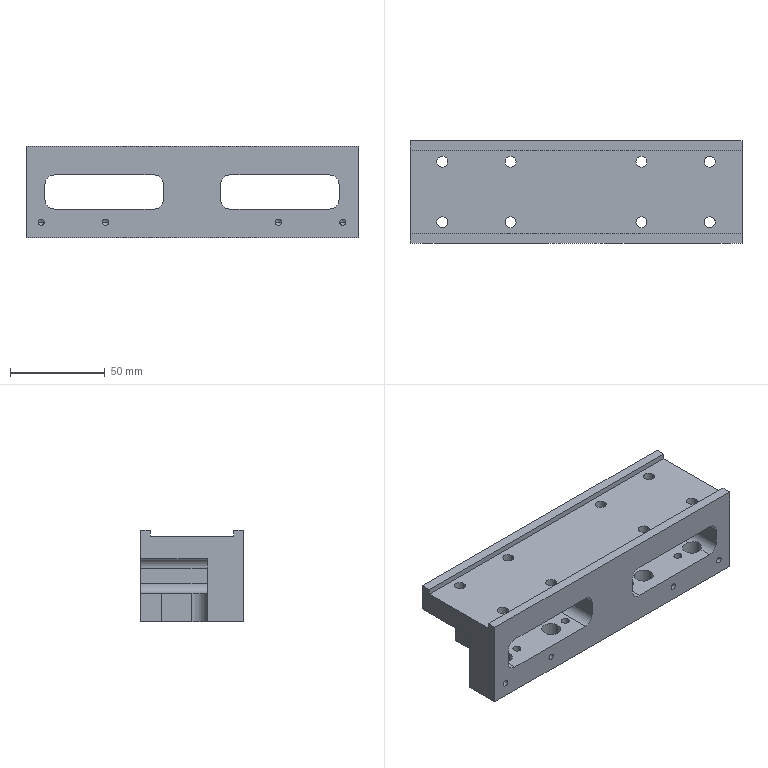Part | 1 solid | 91 faces | box 175 x 54 x 48 mm | volume 278909 mm3 | cylinder 63 | plane 20 | cone 8 | commonest cylinder face diameters 10 x22 4.2 x16 5.8 x16 3.3 x8 16 x1